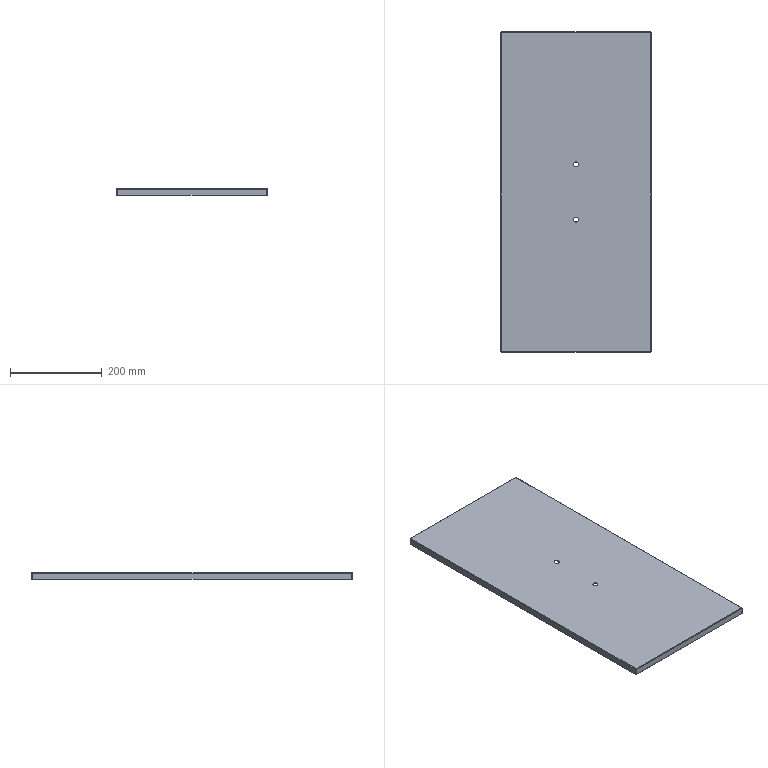Part | SolidWorks | features EdgeFlange 1, FlatPattern 1, ICE 1, SMBaseFlange 1, SheetMetal 1 | 1 solid | 42 faces | box 328.4 x 698.4 x 15 mm | volume 307582 mm3 | plane 22 | cylinder 12 | spline 8 | commonest cylinder face diameters 1 x4 3.4 x4 11 x4